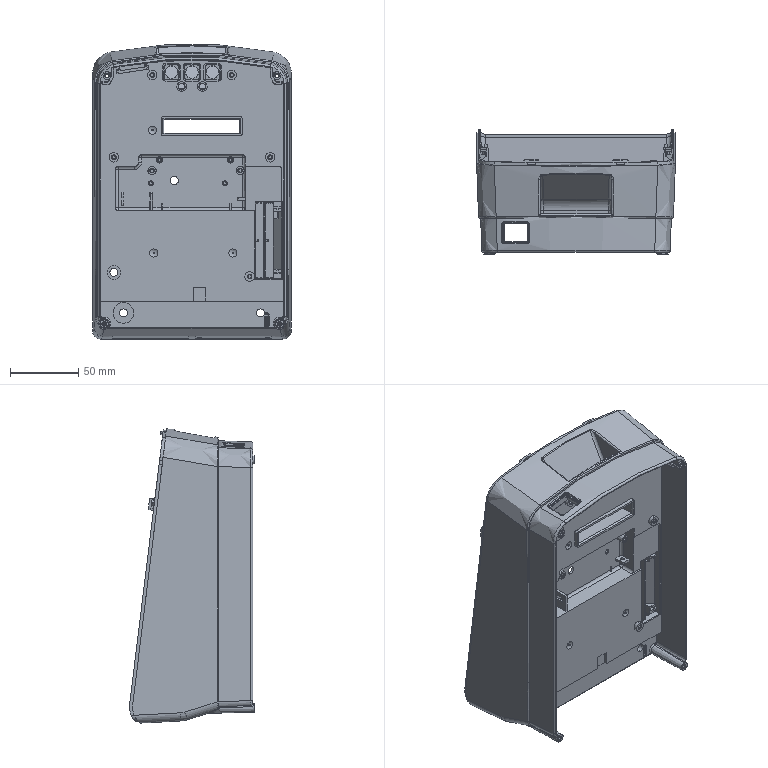Part | STEP file | 6022D002A | 1 solid | 2426 faces | box 145.669 x 91.672 x 216.186 mm | volume 218692 mm3 | plane 1646 | cylinder 305 | spline 263 | cone 142 | torus 34 | sphere 32 | other 4 | commonest cylinder face diameters 1.005 x40 7.035 x32 1.608 x29 2.01 x28 4.02 x28 3.015 x22